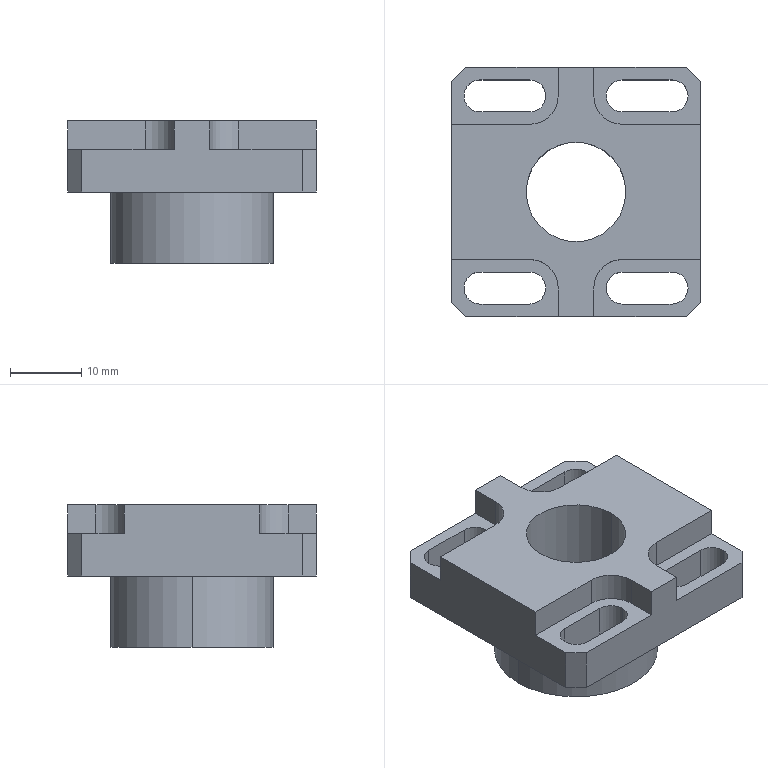Part | STEP file | 08-03 bearing mounting seat | 1 solid | 54 faces | box 35 x 35 x 20 mm | volume 9591 mm3 | plane 32 | cylinder 22 | commonest cylinder face diameters 4.5 x12 8 x4 14 x2 19 x2 22.9 x2